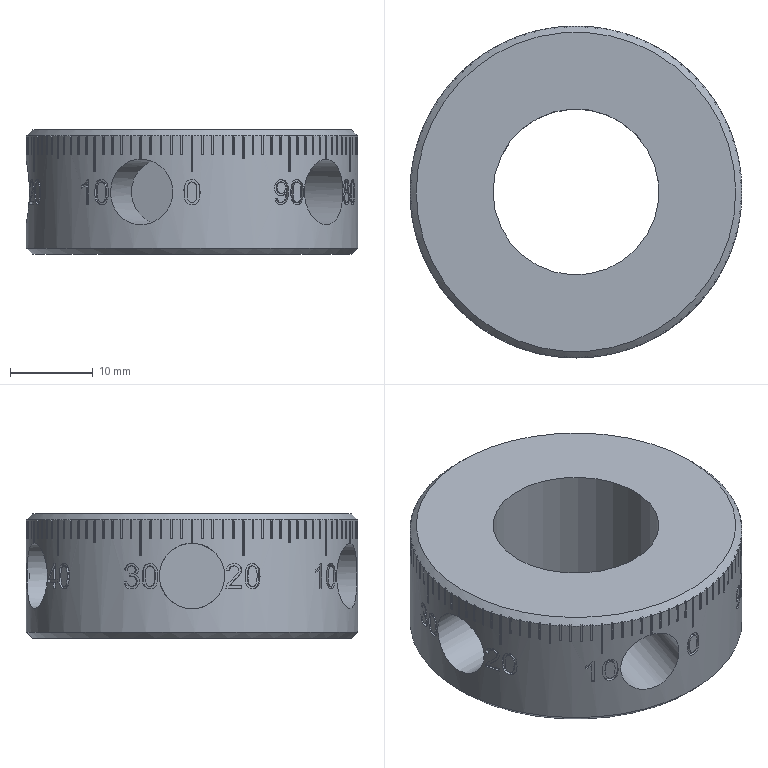Part | STEP file | 冲床-300配套压波_id642_x_t | 1 solid | 533 faces | box 40 x 40 x 15 mm | volume 11990 mm3 | plane 435 | spline 55 | cylinder 41 | cone 2 | commonest cylinder face diameters 39.4 x19 40 x16 7.9 x5 20 x1